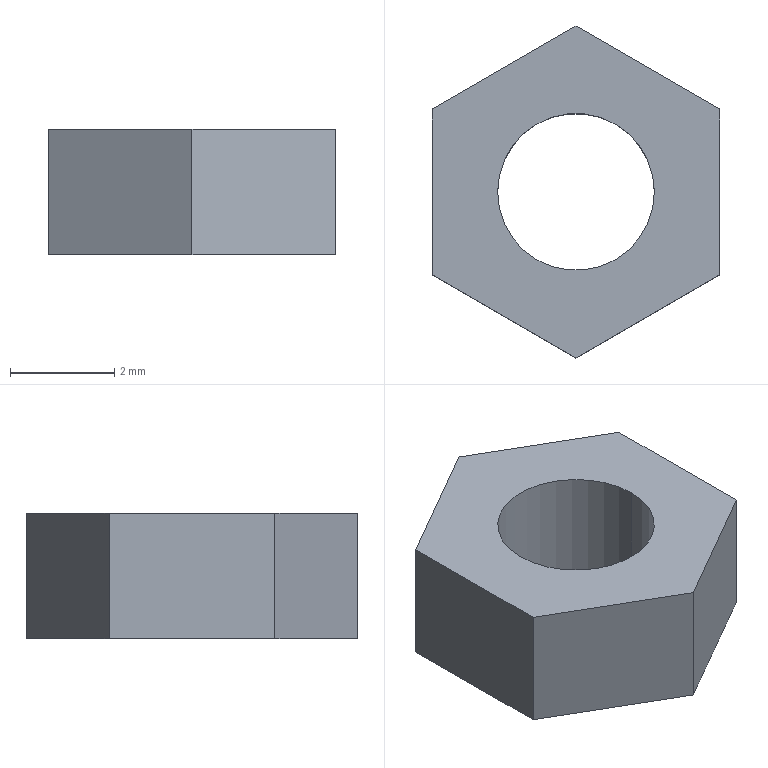Part | STEP file | M3 nut | 1 solid | 10 faces | box 5.5 x 6.351 x 2.4 mm | volume 45.909 mm3 | plane 8 | cylinder 2 | commonest cylinder face diameters 3 x2
STEP:
#1=CARTESIAN_POINT('',(0.,0.,0.));
#2=DIRECTION('',(0.,0.,1.));
#3=DIRECTION('',(1.,0.,0.));
#4=AXIS2_PLACEMENT_3D('',#1,#2,#3);
#5=CARTESIAN_POINT('',(1.5,0.,0.));
#6=VERTEX_POINT('',#5);
#7=CARTESIAN_POINT('',(1.5,0.,2.4));
#8=VERTEX_POINT('',#7);
#9=CARTESIAN_POINT('',(1.5,0.,0.));
#10=DIRECTION('',(0.,0.,1.));
#11=VECTOR('',#10,1.);
#12=LINE('',#9,#11);
#13=CARTESIAN_POINT('',(0.,0.,0.));
#14=DIRECTION('',(0.,0.,1.));
#15=DIRECTION('',(1.,0.,0.));
#16=AXIS2_PLACEMENT_3D('',#13,#14,#15);
#17=CYLINDRICAL_SURFACE('',#16,1.5);
#18=CARTESIAN_POINT('',(6.283,0.));
#19=DIRECTION('',(0.,1.));
#20=VECTOR('',#19,1.);
#21=LINE('',#18,#20);
#22=(GEOMETRIC_REPRESENTATION_CONTEXT(2)PARAMETRIC_REPRESENTATION_CONTEXT()REPRESENTATION_CONTEXT('',''));
#23=DEFINITIONAL_REPRESENTATION('',(#21),#22);
#24=PCURVE('',#17,#23);
#25=CARTESIAN_POINT('',(0.,0.,0.));
#26=DIRECTION('',(0.,0.,1.));
#27=DIRECTION('',(1.,0.,0.));
#28=AXIS2_PLACEMENT_3D('',#25,#26,#27);
#29=CYLINDRICAL_SURFACE('',#28,1.5);
#30=CARTESIAN_POINT('',(0.,0.));
#31=DIRECTION('',(0.,1.));
#32=VECTOR('',#31,1.);
#33=LINE('',#30,#32);
#34=(GEOMETRIC_REPRESENTATION_CONTEXT(2)PARAMETRIC_REPRESENTATION_CONTEXT()REPRESENTATION_CONTEXT('',''));
#35=DEFINITIONAL_REPRESENTATION('',(#33),#34);
#36=PCURVE('',#29,#35);
#37=SURFACE_CURVE('',#12,(#24,#36),.PCURVE_S1.);
#38=EDGE_CURVE('',#6,#8,#37,.T.);
#39=ORIENTED_EDGE('',*,*,#38,.T.);
#40=CARTESIAN_POINT('',(-1.5,0.,2.4));
#41=VERTEX_POINT('',#40);
#42=CARTESIAN_POINT('',(0.,0.,2.4));
#43=DIRECTION('',(0.,0.,1.));
#44=DIRECTION('',(1.,0.,0.));
#45=AXIS2_PLACEMENT_3D('',#42,#43,#44);
#46=CIRCLE('',#45,1.5);
#47=CARTESIAN_POINT('',(0.,2.4));
#48=DIRECTION('',(1.,0.));
#49=VECTOR('',#48,1.);
#50=LINE('',#47,#49);
#51=(GEOMETRIC_REPRESENTATION_CONTEXT(2)PARAMETRIC_REPRESENTATION_CONTEXT()REPRESENTATION_CONTEXT('',''));
#52=DEFINITIONAL_REPRESENTATION('',(#50),#51);
#53=PCURVE('',#17,#52);
#54=CARTESIAN_POINT('',(0.,0.,2.4));
#55=DIRECTION('',(0.,0.,1.));
#56=DIRECTION('',(1.,0.,0.));
#57=AXIS2_PLACEMENT_3D('',#54,#55,#56);
#58=PLANE('',#57);
#59=CARTESIAN_POINT('',(0.,0.));
#60=DIRECTION('',(1.,0.));
#61=AXIS2_PLACEMENT_2D('',#59,#60);
#62=CIRCLE('',#61,1.5);
#63=(GEOMETRIC_REPRESENTATION_CONTEXT(2)PARAMETRIC_REPRESENTATION_CONTEXT()REPRESENTATION_CONTEXT('',''));
#64=DEFINITIONAL_REPRESENTATION('',(#62),#63);
#65=PCURVE('',#58,#64);
#66=SURFACE_CURVE('',#46,(#53,#65),.PCURVE_S1.);
#67=EDGE_CURVE('',#41,#8,#66,.T.);
#68=ORIENTED_EDGE('',*,*,#67,.F.);
#69=CARTESIAN_POINT('',(-1.5,0.,0.));
#70=VERTEX_POINT('',#69);
#71=CARTESIAN_POINT('',(-1.5,0.,0.));
#72=DIRECTION('',(0.,0.,1.));
#73=VECTOR('',#72,1.);
#74=LINE('',#71,#73);
#75=CARTESIAN_POINT('',(3.142,0.));
#76=DIRECTION('',(0.,1.));
#77=VECTOR('',#76,1.);
#78=LINE('',#75,#77);
#79=(GEOMETRIC_REPRESENTATION_CONTEXT(2)PARAMETRIC_REPRESENTATION_CONTEXT()REPRESENTATION_CONTEXT('',''));
#80=DEFINITIONAL_REPRESENTATION('',(#78),#79);
#81=PCURVE('',#17,#80);
#82=CARTESIAN_POINT('',(3.142,0.));
#83=DIRECTION('',(0.,1.));
#84=VECTOR('',#83,1.);
#85=LINE('',#82,#84);
#86=(GEOMETRIC_REPRESENTATION_CONTEXT(2)PARAMETRIC_REPRESENTATION_CONTEXT()REPRESENTATION_CONTEXT('',''));
#87=DEFINITIONAL_REPRESENTATION('',(#85),#86);
#88=PCURVE('',#29,#87);
#89=SURFACE_CURVE('',#74,(#81,#88),.PCURVE_S1.);
#90=EDGE_CURVE('',#70,#41,#89,.T.);
#91=ORIENTED_EDGE('',*,*,#90,.F.);
#92=CARTESIAN_POINT('',(0.,0.,0.));
#93=DIRECTION('',(0.,0.,1.));
#94=DIRECTION('',(1.,0.,0.));
#95=AXIS2_PLACEMENT_3D('',#92,#93,#94);
#96=CIRCLE('',#95,1.5);
#97=CARTESIAN_POINT('',(0.,0.));
#98=DIRECTION('',(1.,0.));
#99=VECTOR('',#98,1.);
#100=LINE('',#97,#99);
#101=(GEOMETRIC_REPRESENTATION_CONTEXT(2)PARAMETRIC_REPRESENTATION_CONTEXT()REPRESENTATION_CONTEXT('',''));
#102=DEFINITIONAL_REPRESENTATION('',(#100),#101);
#103=PCURVE('',#17,#102);
#104=CARTESIAN_POINT('',(0.,0.,0.));
#105=DIRECTION('',(0.,0.,1.));
#106=DIRECTION('',(1.,0.,0.));
#107=AXIS2_PLACEMENT_3D('',#104,#105,#106);
#108=PLANE('',#107);
#109=CARTESIAN_POINT('',(0.,0.));
#110=DIRECTION('',(1.,0.));
#111=AXIS2_PLACEMENT_2D('',#109,#110);
#112=CIRCLE('',#111,1.5);
#113=(GEOMETRIC_REPRESENTATION_CONTEXT(2)PARAMETRIC_REPRESENTATION_CONTEXT()REPRESENTATION_CONTEXT('',''));
#114=DEFINITIONAL_REPRESENTATION('',(#112),#113);
#115=PCURVE('',#108,#114);
#116=SURFACE_CURVE('',#96,(#103,#115),.PCURVE_S1.);
#117=EDGE_CURVE('',#70,#6,#116,.T.);
#118=ORIENTED_EDGE('',*,*,#117,.T.);
#119=EDGE_LOOP('',(#39,#68,#91,#118));
#120=FACE_BOUND('',#119,.F.);
#121=ADVANCED_FACE('',(#120),#17,.F.);
#122=CARTESIAN_POINT('',(-2.75,1.588,0.));
#123=VERTEX_POINT('',#122);
#124=CARTESIAN_POINT('',(-2.75,-1.588,0.));
#125=VERTEX_POINT('',#124);
#126=CARTESIAN_POINT('',(-2.75,1.588,0.));
#127=DIRECTION('',(0.,-1.,0.));
#128=VECTOR('',#127,1.);
#129=LINE('',#126,#128);
#130=CARTESIAN_POINT('',(-2.75,1.588,2.4));
#131=DIRECTION('',(1.,0.,0.));
#132=DIRECTION('',(0.,0.,-1.));
#133=AXIS2_PLACEMENT_3D('',#130,#131,#132);
#134=PLANE('',#133);
#135=CARTESIAN_POINT('',(2.4,0.));
#136=DIRECTION('',(0.,-1.));
#137=VECTOR('',#136,1.);
#138=LINE('',#135,#137);
#139=(GEOMETRIC_REPRESENTATION_CONTEXT(2)PARAMETRIC_REPRESENTATION_CONTEXT()REPRESENTATION_CONTEXT('',''));
#140=DEFINITIONAL_REPRESENTATION('',(#138),#139);
#141=PCURVE('',#134,#140);
#142=CARTESIAN_POINT('',(-2.75,1.588));
#143=DIRECTION('',(0.,-1.));
#144=VECTOR('',#143,1.);
#145=LINE('',#142,#144);
#146=(GEOMETRIC_REPRESENTATION_CONTEXT(2)PARAMETRIC_REPRESENTATION_CONTEXT()REPRESENTATION_CONTEXT('',''));
#147=DEFINITIONAL_REPRESENTATION('',(#145),#146);
#148=PCURVE('',#108,#147);
#149=SURFACE_CURVE('',#129,(#141,#148),.PCURVE_S1.);
#150=EDGE_CURVE('',#123,#125,#149,.T.);
#151=ORIENTED_EDGE('',*,*,#150,.T.);
#152=CARTESIAN_POINT('',(-2.75,-1.588,2.4));
#153=VERTEX_POINT('',#152);
#154=CARTESIAN_POINT('',(-2.75,-1.588,2.4));
#155=DIRECTION('',(0.,0.,-1.));
#156=VECTOR('',#155,1.);
#157=LINE('',#154,#156);
#158=CARTESIAN_POINT('',(0.,-3.175));
#159=DIRECTION('',(1.,0.));
#160=VECTOR('',#159,1.);
#161=LINE('',#158,#160);
#162=(GEOMETRIC_REPRESENTATION_CONTEXT(2)PARAMETRIC_REPRESENTATION_CONTEXT()REPRESENTATION_CONTEXT('',''));
#163=DEFINITIONAL_REPRESENTATION('',(#161),#162);
#164=PCURVE('',#134,#163);
#165=CARTESIAN_POINT('',(-2.75,-1.588,2.4));
#166=DIRECTION('',(0.5,0.866,0.));
#167=DIRECTION('',(-0.866,0.5,0.));
#168=AXIS2_PLACEMENT_3D('',#165,#166,#167);
#169=PLANE('',#168);
#170=CARTESIAN_POINT('',(0.,0.));
#171=DIRECTION('',(0.,-1.));
#172=VECTOR('',#171,1.);
#173=LINE('',#170,#172);
#174=(GEOMETRIC_REPRESENTATION_CONTEXT(2)PARAMETRIC_REPRESENTATION_CONTEXT()REPRESENTATION_CONTEXT('',''));
#175=DEFINITIONAL_REPRESENTATION('',(#173),#174);
#176=PCURVE('',#169,#175);
#177=SURFACE_CURVE('',#157,(#164,#176),.PCURVE_S1.);
#178=EDGE_CURVE('',#153,#125,#177,.T.);
#179=ORIENTED_EDGE('',*,*,#178,.F.);
#180=CARTESIAN_POINT('',(-2.75,1.588,2.4));
#181=VERTEX_POINT('',#180);
#182=CARTESIAN_POINT('',(-2.75,1.588,2.4));
#183=DIRECTION('',(0.,-1.,0.));
#184=VECTOR('',#183,1.);
#185=LINE('',#182,#184);
#186=CARTESIAN_POINT('',(0.,0.));
#187=DIRECTION('',(0.,-1.));
#188=VECTOR('',#187,1.);
#189=LINE('',#186,#188);
#190=(GEOMETRIC_REPRESENTATION_CONTEXT(2)PARAMETRIC_REPRESENTATION_CONTEXT()REPRESENTATION_CONTEXT('',''));
#191=DEFINITIONAL_REPRESENTATION('',(#189),#190);
#192=PCURVE('',#134,#191);
#193=CARTESIAN_POINT('',(-2.75,1.588));
#194=DIRECTION('',(0.,-1.));
#195=VECTOR('',#194,1.);
#196=LINE('',#193,#195);
#197=(GEOMETRIC_REPRESENTATION_CONTEXT(2)PARAMETRIC_REPRESENTATION_CONTEXT()REPRESENTATION_CONTEXT('',''));
#198=DEFINITIONAL_REPRESENTATION('',(#196),#197);
#199=PCURVE('',#58,#198);
#200=SURFACE_CURVE('',#185,(#192,#199),.PCURVE_S1.);
#201=EDGE_CURVE('',#181,#153,#200,.T.);
#202=ORIENTED_EDGE('',*,*,#201,.F.);
#203=CARTESIAN_POINT('',(-2.75,1.588,2.4));
#204=DIRECTION('',(0.,0.,-1.));
#205=VECTOR('',#204,1.);
#206=LINE('',#203,#205);
#207=CARTESIAN_POINT('',(0.,0.));
#208=DIRECTION('',(1.,0.));
#209=VECTOR('',#208,1.);
#210=LINE('',#207,#209);
#211=(GEOMETRIC_REPRESENTATION_CONTEXT(2)PARAMETRIC_REPRESENTATION_CONTEXT()REPRESENTATION_CONTEXT('',''));
#212=DEFINITIONAL_REPRESENTATION('',(#210),#211);
#213=PCURVE('',#134,#212);
#214=CARTESIAN_POINT('',(0.,3.175,2.4));
#215=DIRECTION('',(0.5,-0.866,0.));
#216=DIRECTION('',(0.866,0.5,0.));
#217=AXIS2_PLACEMENT_3D('',#214,#215,#216);
#218=PLANE('',#217);
#219=CARTESIAN_POINT('',(-3.175,0.));
#220=DIRECTION('',(0.,-1.));
#221=VECTOR('',#220,1.);
#222=LINE('',#219,#221);
#223=(GEOMETRIC_REPRESENTATION_CONTEXT(2)PARAMETRIC_REPRESENTATION_CONTEXT()REPRESENTATION_CONTEXT('',''));
#224=DEFINITIONAL_REPRESENTATION('',(#222),#223);
#225=PCURVE('',#218,#224);
#226=SURFACE_CURVE('',#206,(#213,#225),.PCURVE_S1.);
#227=EDGE_CURVE('',#181,#123,#226,.T.);
#228=ORIENTED_EDGE('',*,*,#227,.T.);
#229=EDGE_LOOP('',(#151,#179,#202,#228));
#230=FACE_BOUND('',#229,.T.);
#231=ADVANCED_FACE('',(#230),#134,.F.);
#232=CARTESIAN_POINT('',(0.,-3.175,0.));
#233=VERTEX_POINT('',#232);
#234=CARTESIAN_POINT('',(-2.75,-1.588,0.));
#235=DIRECTION('',(0.866,-0.5,0.));
#236=VECTOR('',#235,1.);
#237=LINE('',#234,#236);
#238=CARTESIAN_POINT('',(0.,-2.4));
#239=DIRECTION('',(-1.,0.));
#240=VECTOR('',#239,1.);
#241=LINE('',#238,#240);
#242=(GEOMETRIC_REPRESENTATION_CONTEXT(2)PARAMETRIC_REPRESENTATION_CONTEXT()REPRESENTATION_CONTEXT('',''));
#243=DEFINITIONAL_REPRESENTATION('',(#241),#242);
#244=PCURVE('',#169,#243);
#245=CARTESIAN_POINT('',(-2.75,-1.588));
#246=DIRECTION('',(0.866,-0.5));
#247=VECTOR('',#246,1.);
#248=LINE('',#245,#247);
#249=(GEOMETRIC_REPRESENTATION_CONTEXT(2)PARAMETRIC_REPRESENTATION_CONTEXT()REPRESENTATION_CONTEXT('',''));
#250=DEFINITIONAL_REPRESENTATION('',(#248),#249);
#251=PCURVE('',#108,#250);
#252=SURFACE_CURVE('',#237,(#244,#251),.PCURVE_S1.);
#253=EDGE_CURVE('',#125,#233,#252,.T.);
#254=ORIENTED_EDGE('',*,*,#253,.T.);
#255=CARTESIAN_POINT('',(0.,-3.175,2.4));
#256=VERTEX_POINT('',#255);
#257=CARTESIAN_POINT('',(0.,-3.175,2.4));
#258=DIRECTION('',(0.,0.,-1.));
#259=VECTOR('',#258,1.);
#260=LINE('',#257,#259);
#261=CARTESIAN_POINT('',(-3.175,0.));
#262=DIRECTION('',(0.,-1.));
#263=VECTOR('',#262,1.);
#264=LINE('',#261,#263);
#265=(GEOMETRIC_REPRESENTATION_CONTEXT(2)PARAMETRIC_REPRESENTATION_CONTEXT()REPRESENTATION_CONTEXT('',''));
#266=DEFINITIONAL_REPRESENTATION('',(#264),#265);
#267=PCURVE('',#169,#266);
#268=CARTESIAN_POINT('',(0.,-3.175,2.4));
#269=DIRECTION('',(-0.5,0.866,0.));
#270=DIRECTION('',(-0.866,-0.5,0.));
#271=AXIS2_PLACEMENT_3D('',#268,#269,#270);
#272=PLANE('',#271);
#273=CARTESIAN_POINT('',(0.,0.));
#274=DIRECTION('',(0.,-1.));
#275=VECTOR('',#274,1.);
#276=LINE('',#273,#275);
#277=(GEOMETRIC_REPRESENTATION_CONTEXT(2)PARAMETRIC_REPRESENTATION_CONTEXT()REPRESENTATION_CONTEXT('',''));
#278=DEFINITIONAL_REPRESENTATION('',(#276),#277);
#279=PCURVE('',#272,#278);
#280=SURFACE_CURVE('',#260,(#267,#279),.PCURVE_S1.);
#281=EDGE_CURVE('',#256,#233,#280,.T.);
#282=ORIENTED_EDGE('',*,*,#281,.F.);
#283=CARTESIAN_POINT('',(-2.75,-1.588,2.4));
#284=DIRECTION('',(0.866,-0.5,0.));
#285=VECTOR('',#284,1.);
#286=LINE('',#283,#285);
#287=CARTESIAN_POINT('',(0.,0.));
#288=DIRECTION('',(-1.,0.));
#289=VECTOR('',#288,1.);
#290=LINE('',#287,#289);
#291=(GEOMETRIC_REPRESENTATION_CONTEXT(2)PARAMETRIC_REPRESENTATION_CONTEXT()REPRESENTATION_CONTEXT('',''));
#292=DEFINITIONAL_REPRESENTATION('',(#290),#291);
#293=PCURVE('',#169,#292);
#294=CARTESIAN_POINT('',(-2.75,-1.588));
#295=DIRECTION('',(0.866,-0.5));
#296=VECTOR('',#295,1.);
#297=LINE('',#294,#296);
#298=(GEOMETRIC_REPRESENTATION_CONTEXT(2)PARAMETRIC_REPRESENTATION_CONTEXT()REPRESENTATION_CONTEXT('',''));
#299=DEFINITIONAL_REPRESENTATION('',(#297),#298);
#300=PCURVE('',#58,#299);
#301=SURFACE_CURVE('',#286,(#293,#300),.PCURVE_S1.);
#302=EDGE_CURVE('',#153,#256,#301,.T.);
#303=ORIENTED_EDGE('',*,*,#302,.F.);
#304=ORIENTED_EDGE('',*,*,#178,.T.);
#305=EDGE_LOOP('',(#254,#282,#303,#304));
#306=FACE_BOUND('',#305,.T.);
#307=ADVANCED_FACE('',(#306),#169,.F.);
#308=CARTESIAN_POINT('',(2.75,-1.588,0.));
#309=VERTEX_POINT('',#308);
#310=CARTESIAN_POINT('',(0.,-3.175,0.));
#311=DIRECTION('',(0.866,0.5,0.));
#312=VECTOR('',#311,1.);
#313=LINE('',#310,#312);
#314=CARTESIAN_POINT('',(0.,-2.4));
#315=DIRECTION('',(-1.,0.));
#316=VECTOR('',#315,1.);
#317=LINE('',#314,#316);
#318=(GEOMETRIC_REPRESENTATION_CONTEXT(2)PARAMETRIC_REPRESENTATION_CONTEXT()REPRESENTATION_CONTEXT('',''));
#319=DEFINITIONAL_REPRESENTATION('',(#317),#318);
#320=PCURVE('',#272,#319);
#321=CARTESIAN_POINT('',(0.,-3.175));
#322=DIRECTION('',(0.866,0.5));
#323=VECTOR('',#322,1.);
#324=LINE('',#321,#323);
#325=(GEOMETRIC_REPRESENTATION_CONTEXT(2)PARAMETRIC_REPRESENTATION_CONTEXT()REPRESENTATION_CONTEXT('',''));
#326=DEFINITIONAL_REPRESENTATION('',(#324),#325);
#327=PCURVE('',#108,#326);
#328=SURFACE_CURVE('',#313,(#320,#327),.PCURVE_S1.);
#329=EDGE_CURVE('',#233,#309,#328,.T.);
#330=ORIENTED_EDGE('',*,*,#329,.T.);
#331=CARTESIAN_POINT('',(2.75,-1.588,2.4));
#332=VERTEX_POINT('',#331);
#333=CARTESIAN_POINT('',(2.75,-1.588,2.4));
#334=DIRECTION('',(0.,0.,-1.));
#335=VECTOR('',#334,1.);
#336=LINE('',#333,#335);
#337=CARTESIAN_POINT('',(-3.175,0.));
#338=DIRECTION('',(0.,-1.));
#339=VECTOR('',#338,1.);
#340=LINE('',#337,#339);
#341=(GEOMETRIC_REPRESENTATION_CONTEXT(2)PARAMETRIC_REPRESENTATION_CONTEXT()REPRESENTATION_CONTEXT('',''));
#342=DEFINITIONAL_REPRESENTATION('',(#340),#341);
#343=PCURVE('',#272,#342);
#344=CARTESIAN_POINT('',(2.75,-1.588,2.4));
#345=DIRECTION('',(-1.,0.,0.));
#346=DIRECTION('',(0.,0.,1.));
#347=AXIS2_PLACEMENT_3D('',#344,#345,#346);
#348=PLANE('',#347);
#349=CARTESIAN_POINT('',(0.,0.));
#350=DIRECTION('',(-1.,0.));
#351=VECTOR('',#350,1.);
#352=LINE('',#349,#351);
#353=(GEOMETRIC_REPRESENTATION_CONTEXT(2)PARAMETRIC_REPRESENTATION_CONTEXT()REPRESENTATION_CONTEXT('',''));
#354=DEFINITIONAL_REPRESENTATION('',(#352),#353);
#355=PCURVE('',#348,#354);
#356=SURFACE_CURVE('',#336,(#343,#355),.PCURVE_S1.);
#357=EDGE_CURVE('',#332,#309,#356,.T.);
#358=ORIENTED_EDGE('',*,*,#357,.F.);
#359=CARTESIAN_POINT('',(0.,-3.175,2.4));
#360=DIRECTION('',(0.866,0.5,0.));
#361=VECTOR('',#360,1.);
#362=LINE('',#359,#361);
#363=CARTESIAN_POINT('',(0.,0.));
#364=DIRECTION('',(-1.,0.));
#365=VECTOR('',#364,1.);
#366=LINE('',#363,#365);
#367=(GEOMETRIC_REPRESENTATION_CONTEXT(2)PARAMETRIC_REPRESENTATION_CONTEXT()REPRESENTATION_CONTEXT('',''));
#368=DEFINITIONAL_REPRESENTATION('',(#366),#367);
#369=PCURVE('',#272,#368);
#370=CARTESIAN_POINT('',(0.,-3.175));
#371=DIRECTION('',(0.866,0.5));
#372=VECTOR('',#371,1.);
#373=LINE('',#370,#372);
#374=(GEOMETRIC_REPRESENTATION_CONTEXT(2)PARAMETRIC_REPRESENTATION_CONTEXT()REPRESENTATION_CONTEXT('',''));
#375=DEFINITIONAL_REPRESENTATION('',(#373),#374);
#376=PCURVE('',#58,#375);
#377=SURFACE_CURVE('',#362,(#369,#376),.PCURVE_S1.);
#378=EDGE_CURVE('',#256,#332,#377,.T.);
#379=ORIENTED_EDGE('',*,*,#378,.F.);
#380=ORIENTED_EDGE('',*,*,#281,.T.);
#381=EDGE_LOOP('',(#330,#358,#379,#380));
#382=FACE_BOUND('',#381,.T.);
#383=ADVANCED_FACE('',(#382),#272,.F.);
#384=CARTESIAN_POINT('',(2.75,1.588,0.));
#385=VERTEX_POINT('',#384);
#386=CARTESIAN_POINT('',(2.75,-1.588,0.));
#387=DIRECTION('',(0.,1.,0.));
#388=VECTOR('',#387,1.);
#389=LINE('',#386,#388);
#390=CARTESIAN_POINT('',(-2.4,0.));
#391=DIRECTION('',(0.,1.));
#392=VECTOR('',#391,1.);
#393=LINE('',#390,#392);
#394=(GEOMETRIC_REPRESENTATION_CONTEXT(2)PARAMETRIC_REPRESENTATION_CONTEXT()REPRESENTATION_CONTEXT('',''));
#395=DEFINITIONAL_REPRESENTATION('',(#393),#394);
#396=PCURVE('',#348,#395);
#397=CARTESIAN_POINT('',(2.75,-1.588));
#398=DIRECTION('',(0.,1.));
#399=VECTOR('',#398,1.);
#400=LINE('',#397,#399);
#401=(GEOMETRIC_REPRESENTATION_CONTEXT(2)PARAMETRIC_REPRESENTATION_CONTEXT()REPRESENTATION_CONTEXT('',''));
#402=DEFINITIONAL_REPRESENTATION('',(#400),#401);
#403=PCURVE('',#108,#402);
#404=SURFACE_CURVE('',#389,(#396,#403),.PCURVE_S1.);
#405=EDGE_CURVE('',#309,#385,#404,.T.);
#406=ORIENTED_EDGE('',*,*,#405,.T.);
#407=CARTESIAN_POINT('',(2.75,1.588,2.4));
#408=VERTEX_POINT('',#407);
#409=CARTESIAN_POINT('',(2.75,1.588,2.4));
#410=DIRECTION('',(0.,0.,-1.));
#411=VECTOR('',#410,1.);
#412=LINE('',#409,#411);
#413=CARTESIAN_POINT('',(0.,3.175));
#414=DIRECTION('',(-1.,0.));
#415=VECTOR('',#414,1.);
#416=LINE('',#413,#415);
#417=(GEOMETRIC_REPRESENTATION_CONTEXT(2)PARAMETRIC_REPRESENTATION_CONTEXT()REPRESENTATION_CONTEXT('',''));
#418=DEFINITIONAL_REPRESENTATION('',(#416),#417);
#419=PCURVE('',#348,#418);
#420=CARTESIAN_POINT('',(2.75,1.588,2.4));
#421=DIRECTION('',(-0.5,-0.866,0.));
#422=DIRECTION('',(0.866,-0.5,0.));
#423=AXIS2_PLACEMENT_3D('',#420,#421,#422);
#424=PLANE('',#423);
#425=CARTESIAN_POINT('',(0.,0.));
#426=DIRECTION('',(0.,-1.));
#427=VECTOR('',#426,1.);
#428=LINE('',#425,#427);
#429=(GEOMETRIC_REPRESENTATION_CONTEXT(2)PARAMETRIC_REPRESENTATION_CONTEXT()REPRESENTATION_CONTEXT('',''));
#430=DEFINITIONAL_REPRESENTATION('',(#428),#429);
#431=PCURVE('',#424,#430);
#432=SURFACE_CURVE('',#412,(#419,#431),.PCURVE_S1.);
#433=EDGE_CURVE('',#408,#385,#432,.T.);
#434=ORIENTED_EDGE('',*,*,#433,.F.);
#435=CARTESIAN_POINT('',(2.75,-1.588,2.4));
#436=DIRECTION('',(0.,1.,0.));
#437=VECTOR('',#436,1.);
#438=LINE('',#435,#437);
#439=CARTESIAN_POINT('',(0.,0.));
#440=DIRECTION('',(0.,1.));
#441=VECTOR('',#440,1.);
#442=LINE('',#439,#441);
#443=(GEOMETRIC_REPRESENTATION_CONTEXT(2)PARAMETRIC_REPRESENTATION_CONTEXT()REPRESENTATION_CONTEXT('',''));
#444=DEFINITIONAL_REPRESENTATION('',(#442),#443);
#445=PCURVE('',#348,#444);
#446=CARTESIAN_POINT('',(2.75,-1.588));
#447=DIRECTION('',(0.,1.));
#448=VECTOR('',#447,1.);
#449=LINE('',#446,#448);
#450=(GEOMETRIC_REPRESENTATION_CONTEXT(2)PARAMETRIC_REPRESENTATION_CONTEXT()REPRESENTATION_CONTEXT('',''));
#451=DEFINITIONAL_REPRESENTATION('',(#449),#450);
#452=PCURVE('',#58,#451);
#453=SURFACE_CURVE('',#438,(#445,#452),.PCURVE_S1.);
#454=EDGE_CURVE('',#332,#408,#453,.T.);
#455=ORIENTED_EDGE('',*,*,#454,.F.);
#456=ORIENTED_EDGE('',*,*,#357,.T.);
#457=EDGE_LOOP('',(#406,#434,#455,#456));
#458=FACE_BOUND('',#457,.T.);
#459=ADVANCED_FACE('',(#458),#348,.F.);
#460=CARTESIAN_POINT('',(0.,3.175,0.));
#461=VERTEX_POINT('',#460);
#462=CARTESIAN_POINT('',(2.75,1.588,0.));
#463=DIRECTION('',(-0.866,0.5,0.));
#464=VECTOR('',#463,1.);
#465=LINE('',#462,#464);
#466=CARTESIAN_POINT('',(0.,-2.4));
#467=DIRECTION('',(-1.,0.));
#468=VECTOR('',#467,1.);
#469=LINE('',#466,#468);
#470=(GEOMETRIC_REPRESENTATION_CONTEXT(2)PARAMETRIC_REPRESENTATION_CONTEXT()REPRESENTATION_CONTEXT('',''));
#471=DEFINITIONAL_REPRESENTATION('',(#469),#470);
#472=PCURVE('',#424,#471);
#473=CARTESIAN_POINT('',(2.75,1.588));
#474=DIRECTION('',(-0.866,0.5));
#475=VECTOR('',#474,1.);
#476=LINE('',#473,#475);
#477=(GEOMETRIC_REPRESENTATION_CONTEXT(2)PARAMETRIC_REPRESENTATION_CONTEXT()REPRESENTATION_CONTEXT('',''));
#478=DEFINITIONAL_REPRESENTATION('',(#476),#477);
#479=PCURVE('',#108,#478);
#480=SURFACE_CURVE('',#465,(#472,#479),.PCURVE_S1.);
#481=EDGE_CURVE('',#385,#461,#480,.T.);
#482=ORIENTED_EDGE('',*,*,#481,.T.);
#483=CARTESIAN_POINT('',(0.,3.175,2.4));
#484=VERTEX_POINT('',#483);
#485=CARTESIAN_POINT('',(0.,3.175,2.4));
#486=DIRECTION('',(0.,0.,-1.));
#487=VECTOR('',#486,1.);
#488=LINE('',#485,#487);
#489=CARTESIAN_POINT('',(-3.175,0.));
#490=DIRECTION('',(0.,-1.));
#491=VECTOR('',#490,1.);
#492=LINE('',#489,#491);
#493=(GEOMETRIC_REPRESENTATION_CONTEXT(2)PARAMETRIC_REPRESENTATION_CONTEXT()REPRESENTATION_CONTEXT('',''));
#494=DEFINITIONAL_REPRESENTATION('',(#492),#493);
#495=PCURVE('',#424,#494);
#496=CARTESIAN_POINT('',(0.,0.));
#497=DIRECTION('',(0.,-1.));
#498=VECTOR('',#497,1.);
#499=LINE('',#496,#498);
#500=(GEOMETRIC_REPRESENTATION_CONTEXT(2)PARAMETRIC_REPRESENTATION_CONTEXT()REPRESENTATION_CONTEXT('',''));
#501=DEFINITIONAL_REPRESENTATION('',(#499),#500);
#502=PCURVE('',#218,#501);
#503=SURFACE_CURVE('',#488,(#495,#502),.PCURVE_S1.);
#504=EDGE_CURVE('',#484,#461,#503,.T.);
#505=ORIENTED_EDGE('',*,*,#504,.F.);
#506=CARTESIAN_POINT('',(2.75,1.588,2.4));
#507=DIRECTION('',(-0.866,0.5,0.));
#508=VECTOR('',#507,1.);
#509=LINE('',#506,#508);
#510=CARTESIAN_POINT('',(0.,0.));
#511=DIRECTION('',(-1.,0.));
#512=VECTOR('',#511,1.);
#513=LINE('',#510,#512);
#514=(GEOMETRIC_REPRESENTATION_CONTEXT(2)PARAMETRIC_REPRESENTATION_CONTEXT()REPRESENTATION_CONTEXT('',''));
#515=DEFINITIONAL_REPRESENTATION('',(#513),#514);
#516=PCURVE('',#424,#515);
#517=CARTESIAN_POINT('',(2.75,1.588));
#518=DIRECTION('',(-0.866,0.5));
#519=VECTOR('',#518,1.);
#520=LINE('',#517,#519);
#521=(GEOMETRIC_REPRESENTATION_CONTEXT(2)PARAMETRIC_REPRESENTATION_CONTEXT()REPRESENTATION_CONTEXT('',''));
#522=DEFINITIONAL_REPRESENTATION('',(#520),#521);
#523=PCURVE('',#58,#522);
#524=SURFACE_CURVE('',#509,(#516,#523),.PCURVE_S1.);
#525=EDGE_CURVE('',#408,#484,#524,.T.);
#526=ORIENTED_EDGE('',*,*,#525,.F.);
#527=ORIENTED_EDGE('',*,*,#433,.T.);
#528=EDGE_LOOP('',(#482,#505,#526,#527));
#529=FACE_BOUND('',#528,.T.);
#530=ADVANCED_FACE('',(#529),#424,.F.);
#531=CARTESIAN_POINT('',(0.,3.175,0.));
#532=DIRECTION('',(-0.866,-0.5,0.));
#533=VECTOR('',#532,1.);
#534=LINE('',#531,#533);
#535=CARTESIAN_POINT('',(0.,-2.4));
#536=DIRECTION('',(-1.,0.));
#537=VECTOR('',#536,1.);
#538=LINE('',#535,#537);
#539=(GEOMETRIC_REPRESENTATION_CONTEXT(2)PARAMETRIC_REPRESENTATION_CONTEXT()REPRESENTATION_CONTEXT('',''));
#540=DEFINITIONAL_REPRESENTATION('',(#538),#539);
#541=PCURVE('',#218,#540);
#542=CARTESIAN_POINT('',(0.,3.175));
#543=DIRECTION('',(-0.866,-0.5));
#544=VECTOR('',#543,1.);
#545=LINE('',#542,#544);
#546=(GEOMETRIC_REPRESENTATION_CONTEXT(2)PARAMETRIC_REPRESENTATION_CONTEXT()REPRESENTATION_CONTEXT('',''));
#547=DEFINITIONAL_REPRESENTATION('',(#545),#546);
#548=PCURVE('',#108,#547);
#549=SURFACE_CURVE('',#534,(#541,#548),.PCURVE_S1.);
#550=EDGE_CURVE('',#461,#123,#549,.T.);
#551=ORIENTED_EDGE('',*,*,#550,.T.);
#552=ORIENTED_EDGE('',*,*,#227,.F.);
#553=CARTESIAN_POINT('',(0.,3.175,2.4));
#554=DIRECTION('',(-0.866,-0.5,0.));
#555=VECTOR('',#554,1.);
#556=LINE('',#553,#555);
#557=CARTESIAN_POINT('',(0.,0.));
#558=DIRECTION('',(-1.,0.));
#559=VECTOR('',#558,1.);
#560=LINE('',#557,#559);
#561=(GEOMETRIC_REPRESENTATION_CONTEXT(2)PARAMETRIC_REPRESENTATION_CONTEXT()REPRESENTATION_CONTEXT('',''));
#562=DEFINITIONAL_REPRESENTATION('',(#560),#561);
#563=PCURVE('',#218,#562);
#564=CARTESIAN_POINT('',(0.,3.175));
#565=DIRECTION('',(-0.866,-0.5));
#566=VECTOR('',#565,1.);
#567=LINE('',#564,#566);
#568=(GEOMETRIC_REPRESENTATION_CONTEXT(2)PARAMETRIC_REPRESENTATION_CONTEXT()REPRESENTATION_CONTEXT('',''));
#569=DEFINITIONAL_REPRESENTATION('',(#567),#568);
#570=PCURVE('',#58,#569);
#571=SURFACE_CURVE('',#556,(#563,#570),.PCURVE_S1.);
#572=EDGE_CURVE('',#484,#181,#571,.T.);
#573=ORIENTED_EDGE('',*,*,#572,.F.);
#574=ORIENTED_EDGE('',*,*,#504,.T.);
#575=EDGE_LOOP('',(#551,#552,#573,#574));
#576=FACE_BOUND('',#575,.T.);
#577=ADVANCED_FACE('',(#576),#218,.F.);
#578=CARTESIAN_POINT('',(0.,0.,2.4));
#579=DIRECTION('',(0.,0.,1.));
#580=DIRECTION('',(1.,0.,0.));
#581=AXIS2_PLACEMENT_3D('',#578,#579,#580);
#582=CIRCLE('',#581,1.5);
#583=CARTESIAN_POINT('',(0.,0.));
#584=DIRECTION('',(1.,0.));
#585=AXIS2_PLACEMENT_2D('',#583,#584);
#586=CIRCLE('',#585,1.5);
#587=(GEOMETRIC_REPRESENTATION_CONTEXT(2)PARAMETRIC_REPRESENTATION_CONTEXT()REPRESENTATION_CONTEXT('',''));
#588=DEFINITIONAL_REPRESENTATION('',(#586),#587);
#589=PCURVE('',#58,#588);
#590=CARTESIAN_POINT('',(0.,2.4));
#591=DIRECTION('',(1.,0.));
#592=VECTOR('',#591,1.);
#593=LINE('',#590,#592);
#594=(GEOMETRIC_REPRESENTATION_CONTEXT(2)PARAMETRIC_REPRESENTATION_CONTEXT()REPRESENTATION_CONTEXT('',''));
#595=DEFINITIONAL_REPRESENTATION('',(#593),#594);
#596=PCURVE('',#29,#595);
#597=SURFACE_CURVE('',#582,(#589,#596),.PCURVE_S1.);
#598=EDGE_CURVE('',#8,#41,#597,.T.);
#599=ORIENTED_EDGE('',*,*,#598,.F.);
#600=ORIENTED_EDGE('',*,*,#67,.F.);
#601=EDGE_LOOP('',(#599,#600));
#602=FACE_BOUND('',#601,.T.);
#603=ORIENTED_EDGE('',*,*,#201,.T.);
#604=ORIENTED_EDGE('',*,*,#302,.T.);
#605=ORIENTED_EDGE('',*,*,#378,.T.);
#606=ORIENTED_EDGE('',*,*,#454,.T.);
#607=ORIENTED_EDGE('',*,*,#525,.T.);
#608=ORIENTED_EDGE('',*,*,#572,.T.);
#609=EDGE_LOOP('',(#603,#604,#605,#606,#607,#608));
#610=FACE_BOUND('',#609,.T.);
#611=ADVANCED_FACE('',(#602,#610),#58,.T.);
#612=CARTESIAN_POINT('',(0.,0.,0.));
#613=DIRECTION('',(0.,0.,1.));
#614=DIRECTION('',(1.,0.,0.));
#615=AXIS2_PLACEMENT_3D('',#612,#613,#614);
#616=CIRCLE('',#615,1.5);
#617=CARTESIAN_POINT('',(0.,0.));
#618=DIRECTION('',(1.,0.));
#619=AXIS2_PLACEMENT_2D('',#617,#618);
#620=CIRCLE('',#619,1.5);
#621=(GEOMETRIC_REPRESENTATION_CONTEXT(2)PARAMETRIC_REPRESENTATION_CONTEXT()REPRESENTATION_CONTEXT('',''));
#622=DEFINITIONAL_REPRESENTATION('',(#620),#621);
#623=PCURVE('',#108,#622);
#624=CARTESIAN_POINT('',(0.,0.));
#625=DIRECTION('',(1.,0.));
#626=VECTOR('',#625,1.);
#627=LINE('',#624,#626);
#628=(GEOMETRIC_REPRESENTATION_CONTEXT(2)PARAMETRIC_REPRESENTATION_CONTEXT()REPRESENTATION_CONTEXT('',''));
#629=DEFINITIONAL_REPRESENTATION('',(#627),#628);
#630=PCURVE('',#29,#629);
#631=SURFACE_CURVE('',#616,(#623,#630),.PCURVE_S1.);
#632=EDGE_CURVE('',#6,#70,#631,.T.);
#633=ORIENTED_EDGE('',*,*,#632,.T.);
#634=ORIENTED_EDGE('',*,*,#117,.T.);
#635=EDGE_LOOP('',(#633,#634));
#636=FACE_BOUND('',#635,.T.);
#637=ORIENTED_EDGE('',*,*,#150,.F.);
#638=ORIENTED_EDGE('',*,*,#550,.F.);
#639=ORIENTED_EDGE('',*,*,#481,.F.);
#640=ORIENTED_EDGE('',*,*,#405,.F.);
#641=ORIENTED_EDGE('',*,*,#329,.F.);
#642=ORIENTED_EDGE('',*,*,#253,.F.);
#643=EDGE_LOOP('',(#637,#638,#639,#640,#641,#642));
#644=FACE_BOUND('',#643,.T.);
#645=ADVANCED_FACE('',(#636,#644),#108,.F.);
#646=ORIENTED_EDGE('',*,*,#598,.F.);
#647=ORIENTED_EDGE('',*,*,#38,.F.);
#648=ORIENTED_EDGE('',*,*,#632,.T.);
#649=ORIENTED_EDGE('',*,*,#90,.T.);
#650=EDGE_LOOP('',(#646,#647,#648,#649));
#651=FACE_BOUND('',#650,.F.);
#652=ADVANCED_FACE('',(#651),#29,.F.);
#653=CLOSED_SHELL('',(#121,#231,#307,#383,#459,#530,#577,#611,#645,#652));
#654=MANIFOLD_SOLID_BREP('',#653);
#655=(LENGTH_UNIT()NAMED_UNIT(*)SI_UNIT(.MILLI.,.METRE.));
#656=UNCERTAINTY_MEASURE_WITH_UNIT(LENGTH_MEASURE(0.0000001),#655,'','');
#657=(NAMED_UNIT(*)PLANE_ANGLE_UNIT()SI_UNIT($,.RADIAN.));
#658=(NAMED_UNIT(*)SI_UNIT($,.STERADIAN.)SOLID_ANGLE_UNIT());
#659=(GEOMETRIC_REPRESENTATION_CONTEXT(3)GLOBAL_UNCERTAINTY_ASSIGNED_CONTEXT((#656))GLOBAL_UNIT_ASSIGNED_CONTEXT((#655,#657,#658))REPRESENTATION_CONTEXT('',''));
#660=ADVANCED_BREP_SHAPE_REPRESENTATION('',(#4,#654),#659);